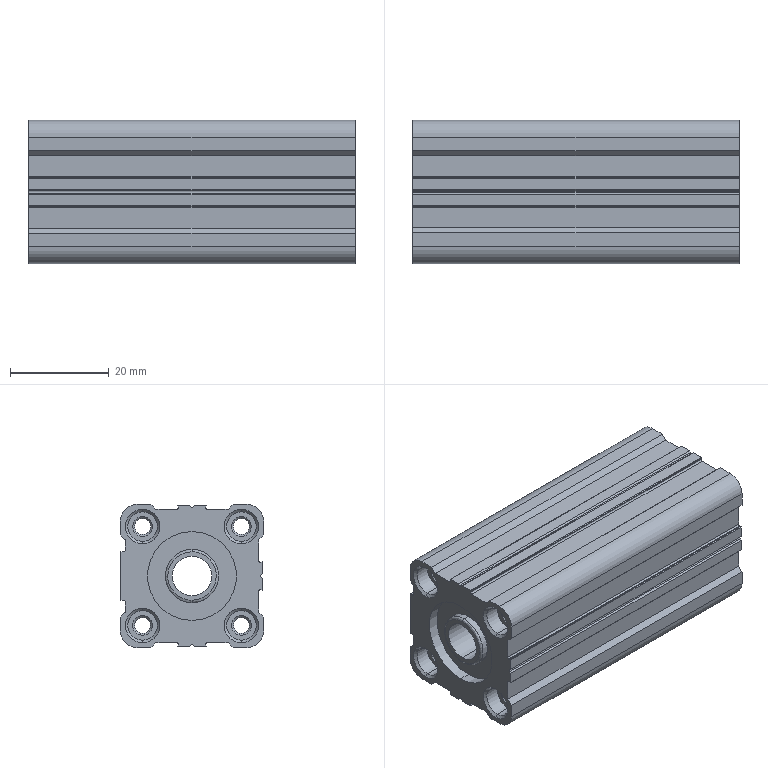Part | STEP file | _ACQJ-16x40-B_b (40) | 1 solid | 173 faces | box 66 x 29 x 29 mm | volume 38011 mm3 | cylinder 70 | plane 63 | cone 36 | spline 4 | commonest cylinder face diameters 6 x16 0.6 x15 0.2 x9 3.242 x8 4.134 x4 6.8 x4